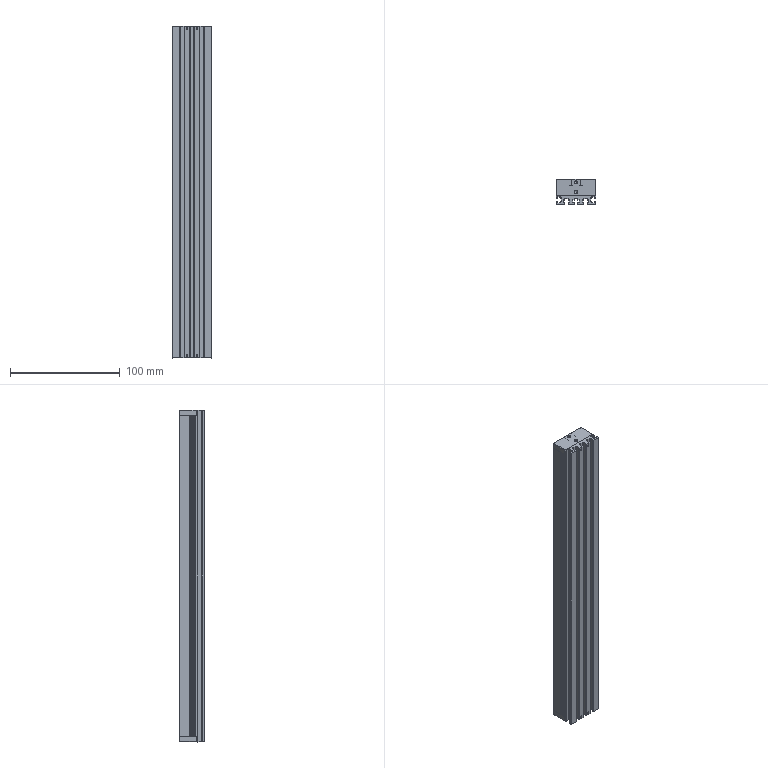Part | SolidWorks | 15 solids | 2059 faces | box 36 x 22.6 x 302 mm | volume 86992 mm3 | spline 720 | plane 601 | cylinder 558 | cone 180 | commonest cylinder face diameters 2 x290 1.9 x144 0.2 x66 0.6 x24 1.6 x10 2.2 x8